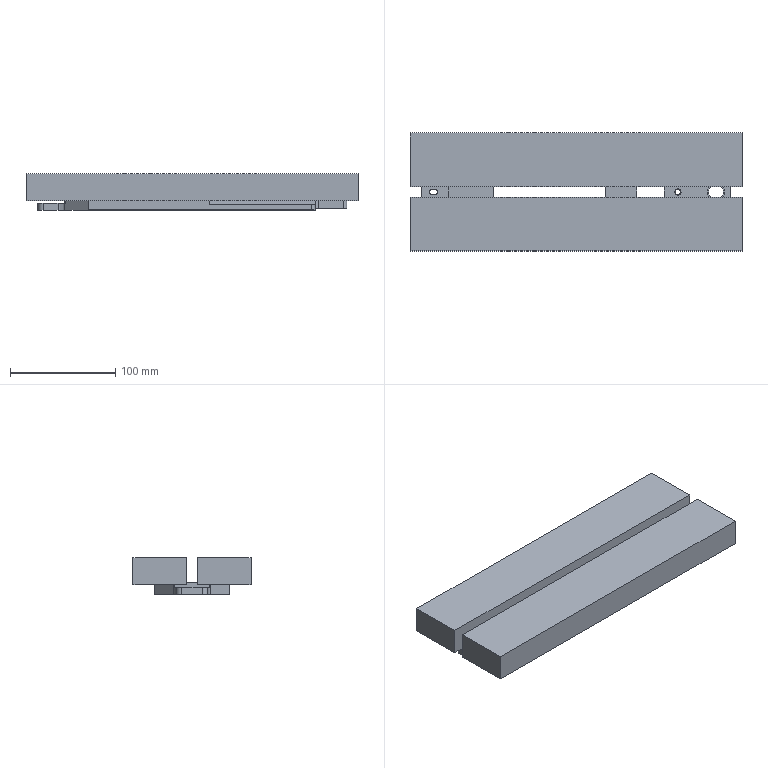NC program | NX | posted with a generic post | part box 315 x 112 x 34.85 mm
Lines 19 to 805 of 11462:
(ADAPTIVE_MILLING , TOOL : D12_ROUGH)
N36 T02 M6
N38 G53
N40 G17 G0 G90 X-161.022 Y-0.963 S6500 M3
N42 G43 Z20. H2
N44 Z-9.
N46 G94 G1 X-160.872 Y-0.957 Z-9.937 F3000.
N48 X-160.722 Y-0.951 Z-10.308
N50 X-160.573 Y-0.945 Z-10.58
N52 X-160.423 Y-0.938 Z-10.8
N54 X-160.273 Y-0.932 Z-10.984
N56 X-160.123 Y-0.926 Z-11.142
N58 X-159.973 Y-0.92 Z-11.28
N60 X-159.823 Y-0.914 Z-11.4
N62 X-159.673 Y-0.908 Z-11.505
N64 X-159.523 Y-0.902 Z-11.598
N66 X-159.374 Y-0.896 Z-11.679
N68 X-159.224 Y-0.89 Z-11.75
N70 X-159.074 Y-0.884 Z-11.81
N72 X-158.924 Y-0.878 Z-11.862
N74 X-158.774 Y-0.872 Z-11.905
N76 X-158.624 Y-0.866 Z-11.939
N78 X-158.474 Y-0.86 Z-11.966
N80 X-158.324 Y-0.854 Z-11.985
N82 X-158.174 Y-0.848 Z-11.996
N84 X-158.025 Y-0.841 Z-12.
N86 X-156.085 Y-0.763
N88 G3 X-155.024 Y-0.037 R1.213
N90 X-154.336 Y3.017 R10.296
N92 X-154.027 Y11.039 R88.268
N94 G1 X-154. Y21.799
N96 G2 X-153.983 Y34.698 R955.634
N98 X-151.786 Y38.926 R6.62
N100 X-146.976 Y41.449 R11.386
N102 X-140.748 Y42.318 R29.799
N104 X-129.951 Y42.495 R232.185
N106 G1 X-123.876 Y42.499
N108 X145.801
N110 G2 X150.265 Y40.486 R6.406
N112 X152.872 Y35.821 R10.892
N114 X153.805 Y29.604 R27.845
N116 X153.995 Y18.207 R225.691
N118 G1 X153.999 Y11.907
N120 X153.998 Y-34.397
N122 G2 X152.106 Y-38.609 R6.376
N124 X147.432 Y-41.316 R10.781
N126 X141.298 Y-42.286 R26.839
N128 X131.476 Y-42.491 R179.768
N130 G1 X123.676 Y-42.499
N132 X-145.826
N134 G2 X-150.172 Y-40.545 R6.379
N136 X-152.866 Y-35.766 R10.949
N138 X-153.801 Y-29.549 R28.01
N140 X-153.994 Y-18.452 R216.598
N142 G1 X-153.999 Y-11.852
N144 X-153.994 Y5.173
N146 G3 X-153.531 Y7.081 R26.231
N148 X-153.077 Y13.66 R49.097
N150 X-152.995 Y31.248 R994.194
N152 G2 X-149.634 Y37.786 R8.754
N154 X-144.116 Y40.403 R14.134
N156 X-136.986 Y41.318 R36.897
N158 X-125.588 Y41.494 R265.971
N160 G1 X-118.988 Y41.499
N162 X-101.337 Y41.5
N164 G3 X-100.411 Y41.826 R2.513
N166 G2 X-98.289 Y42.2 R7.215
N168 G1 X113.711
N170 G2 X116.146 Y41.913 R16.672
N172 G3 X123.066 Y41.545 R62.209
N174 X134.549 Y41.5 R762.557
N176 G2 X143.098 Y41.478 R421.327
N178 X149.417 Y37.997 R8.784
N180 X151.94 Y32.519 R14.268
N182 X152.827 Y25.385 R37.632
N184 X152.995 Y13.987 R280.87
N186 G1 X152.999 Y7.537
N188 X152.997 Y-31.097
N190 G2 X149.622 Y-37.794 R8.752
N192 X144.165 Y-40.39 R14.095
N194 X137.186 Y-41.307 R36.049
N196 X125.339 Y-41.495 R261.794
N198 G1 X117.234 Y-41.511
N200 G3 X116.552 Y-41.75 R3.128
N202 G1 X115.148 Y-42.087
N204 X113.709 Y-42.2
N206 X-98.291
N208 G2 X-100.613 Y-41.898 R21.67
N210 G3 X-107.857 Y-41.539 R67.61
N212 X-119.648 Y-41.5 R794.19
N214 G1 X-142.598 Y-41.498
N216 G2 X-149.284 Y-38.134 R8.75
N218 X-151.91 Y-32.588 R14.151
N220 X-152.811 Y-25.607 R36.598
N222 X-152.993 Y-13.609 R266.033
N224 G1 X-152.999 Y-5.436
N226 G2 X-152.983 Y5.288 R824.874
N228 G3 X-152.49 Y8.476 R39.918
N230 G2 X-152.282 Y12.508 R32.054
N232 G3 X-152.013 Y22.941 R161.961
N234 G2 X-151.969 Y29.075 R201.235
N236 X-147.423 Y36.996 R10.241
N238 X-141.273 Y39.506 R16.877
N240 X-133.453 Y40.345 R46.527
N242 X-118.379 Y40.497 R441.147
N244 G1 X-104.482 Y40.499
N246 G3 X-102.594 Y40.604 R9.216
N248 G1 X-102.277 Y40.748
N250 X-101.391 Y41.369
N252 X-100.847 Y41.622
N254 X-101.391 Y41.369
N256 X-102.395 Y40.654
N258 G2 X-104.258 Y40.192 R5.664
N260 X-110.273 Y39.925 R60.091
N262 G1 X-122.296 Y39.893
N264 G3 X-134.742 Y39.652 R226.868
N266 X-141.852 Y38.604 R34.814
N268 X-147.29 Y35.841 R13.828
N270 X-150.634 Y30.1 R10.73
N272 X-151.308 Y24.374 R29.753
N274 G1 X-151.541 Y15.592
N276 G2 X-151.657 Y14.023 R9.013
N278 G1 X-152.036 Y13.006
N280 X-152.376 Y11.445
N282 X-152.036 Y13.006
N284 G3 X-151.14 Y15.544 R26.474
N286 X-150.538 Y20.465 R29.953
N288 G2 X-150.088 Y26.488 R95.136
N290 X-148.485 Y31.606 R13.365
N292 X-143.036 Y36.419 R12.237
N294 X-136.411 Y38.255 R22.856
N296 X-127.209 Y38.83 R78.815
N298 X-112.541 Y38.913 R971.754
N300 G3 X-105.643 Y39.159 R77.798
N302 X-103.833 Y39.497 R7.727
N304 G1 X-103.609 Y39.629
N306 X-102.288 Y40.739
N308 X-103.782 Y39.486
N310 G2 X-106.184 Y38.756 R6.946
N312 X-112.131 Y38.357 R46.238
N314 X-124.112 Y38.266 R885.684
N316 G3 X-134.15 Y37.857 R115.617
N318 X-140.954 Y36.411 R27.013
N320 X-146.538 Y32.482 R12.6
N322 X-149.081 Y26.769 R14.053
N324 X-149.811 Y21.498 R42.908
N326 G2 X-150.46 Y16.404 R43.199
N328 X-150.711 Y15.906 R1.666
N330 G1 X-151.477 Y14.504
N332 G2 X-150.638 Y16.004 R41.838
N334 G3 X-149.656 Y18.125 R5.692
N336 X-148.735 Y22.918 R47.362
N338 G2 X-147.392 Y28.059 R22.945
N340 X-141.192 Y34.538 R12.717
N342 X-134.538 Y36.537 R22.541
N344 X-125.944 Y37.192 R68.234
N346 X-114.014 Y37.336 R873.961
N348 G3 X-107.369 Y37.716 R57.477
N350 X-105.436 Y38.141 R9.034
N352 G1 X-105.243 Y38.256
N354 X-103.693 Y39.559
N356 X-105.417 Y38.113
N358 G2 X-107.843 Y37.298 R7.378
N360 X-113.764 Y36.79 R40.561
N362 X-124.598 Y36.614 R979.351
N364 G3 X-133.72 Y35.975 R73.644
N366 X-140.245 Y34.068 R22.198
N368 X-146.804 Y26.818 R13.13
N370 X-148.17 Y21.984 R31.33
N372 G2 X-149.256 Y17.819 R31.098
N374 X-149.754 Y17.185 R1.887
N376 G1 X-150.428 Y16.285
N378 G2 X-149.222 Y17.717 R8.221
N380 G3 X-147.996 Y20.064 R7.784
N382 G1 X-146.551 Y24.357
N384 G2 X-143.095 Y30.049 R15.346
N386 X-136.543 Y33.915 R16.052
N388 X-128.886 Y35.307 R34.155
N390 X-118.44 Y35.694 R161.697
N392 G3 X-110.514 Y36.039 R97.198
N394 X-107.222 Y36.656 R16.366
N396 G1 X-106.977 Y36.8
N398 X-105.312 Y38.199
N400 X-107.15 Y36.655
N402 G2 X-109.534 Y35.806 R7.243
N404 X-115.614 Y35.204 R38.765
N406 G3 X-125.866 Y34.878 R827.539
N408 X-133.895 Y33.886 R46.492
N410 X-140.41 Y31.103 R18.239
N412 X-145.287 Y25.101 R15.22
N414 X-147.185 Y20.525 R86.69
N416 G2 X-148.076 Y18.757 R8.533
N418 X-148.624 Y18.315 R6.705
N420 G1 X-149.26 Y17.679
N422 G2 X-147.909 Y18.85 R7.268
N424 G3 X-146.384 Y20.934 R8.025
N426 G2 X-144.143 Y24.995 R97.092
N428 X-135.465 Y31.971 R16.466
N430 X-127.777 Y33.595 R31.965
N432 X-118.897 Y34.088 R132.138
N434 G3 X-111.512 Y34.594 R71.126
N436 X-108.974 Y35.163 R11.718
N438 G1 X-108.784 Y35.282
N440 X-107.118 Y36.681
N442 X-108.956 Y35.137
N444 G2 X-111.543 Y34.22 R7.716
N446 X-117.412 Y33.59 R41.28
N448 G3 X-126.419 Y33.083 R246.05
N450 X-133.999 Y31.676 R35.118
N452 X-143.411 Y24.566 R17.194
N454 X-145.825 Y20.732 R347.167
N456 G2 X-146.652 Y19.668 R5.476
N458 G3 X-147.945 Y18.823 R9.081
N460 G2 X-146.373 Y19.803 R8.108
N462 G3 X-144.494 Y21.681 R9.23
N464 G2 X-141.394 Y25.413 R57.726
N466 X-132.404 Y30.763 R19.687
N468 X-124.284 Y32.138 R41.416
N470 X-116.487 Y32.665 R806.55
N472 G3 X-111.216 Y33.467 R28.558
N474 X-110.647 Y33.717 R1.934
N476 G1 X-108.924 Y35.164
N478 X-110.82 Y33.572
N480 G2 X-113.402 Y32.638 R7.835
N482 X-119.041 Y31.934 R43.599
N484 G3 X-127.086 Y31.181 R120.7
N486 X-134.803 Y29.075 R28.367
N488 X-141.698 Y23.911 R20.858
N490 G2 X-144.537 Y20.793 R86.711
N492 X-145.104 Y20.35 R2.371
N494 G3 X-146.402 Y19.787 R6.455
N496 G2 X-145.104 Y20.35 R6.455
N498 G3 X-143.117 Y21.543 R6.138
N500 G1 X-139.682 Y24.517
N502 G2 X-129.256 Y29.545 R24.551
N504 X-121.918 Y30.642 R57.45
N506 G3 X-115.156 Y31.408 R98.281
N508 X-112.724 Y32.008 R11.913
N510 G1 X-112.559 Y32.111
N512 X-110.778 Y33.607
N514 X-112.731 Y31.967
N516 G2 X-115.4 Y30.983 R8.377
N518 X-120.441 Y30.222 R49.586
N520 G3 X-128.154 Y29.094 R76.929
N522 X-139.68 Y23.566 R26.047
N524 G2 X-142.988 Y20.998 R48.613
N526 G1 X-143.332 Y20.838
N528 G3 X-144.725 Y20.492 R8.423
N530 G2 X-143.332 Y20.838 R8.423
N532 G3 X-140.989 Y21.802 R6.926
N534 G2 X-136.677 Y24.486 R530.565
N536 X-126.061 Y28.318 R32.292
N538 X-118.695 Y29.435 R205.643
N540 G3 X-114.764 Y30.311 R22.958
N542 G1 X-114.557 Y30.433
N544 X-112.719 Y31.977
N546 X-114.73 Y30.29
N548 G2 X-117.28 Y29.292 R8.527
N550 X-122.8 Y28.261 R69.878
N552 G3 X-130.822 Y26.376 R47.603
N554 X-137.85 Y22.977 R36.48
N556 G2 X-141.257 Y21.1 R31.406
N558 G1 X-141.534 Y21.033
N560 X-142.883 Y20.936
N562 G3 X-140.773 Y21.099 R41.743
N564 X-137.648 Y22.245 R14.378
N566 G2 X-131.303 Y25.008 R69.885
N568 X-123.029 Y27.133 R53.867
N570 G3 X-117.436 Y28.347 R59.208
N572 X-116.669 Y28.659 R2.7
N574 G1 X-114.659 Y30.347
N576 X-116.841 Y28.514
N578 G2 X-119.52 Y27.412 R9.596
N580 X-125.615 Y25.979 R178.227
N582 G3 X-135.451 Y22.562 R51.022
N584 G2 X-139.179 Y21.07 R30.883
N586 X-141.202 Y21.05 R28.659
N588 G1 X-138.421 Y21.061
N590 G3 X-135.162 Y21.879 R15.354
N592 G2 X-127.95 Y24.252 R132.533
N594 X-120.997 Y26.028 R482.695
N596 G3 X-119.111 Y26.637 R16.872
N598 G1 X-118.974 Y26.723
N600 X-116.791 Y28.556
N602 G2 X-119.316 Y26.461 R56.651
N604 X-122.413 Y25.198 R13.576
N606 G3 X-129.696 Y23.073 R400.204
N608 G2 X-135.631 Y21.151 R202.756
N610 G1 X-136.109 Y21.05
N612 X-138.584
N614 G3 X-134.618 Y21.07 R118.289
N616 X-130.3 Y21.97 R27.955
N618 X-122.5 Y24.192 R158.808
N620 X-121.482 Y24.616 R4.148
N622 G1 X-119.127 Y26.594
N624 G2 X-121.835 Y24.341 R355.257
N626 X-124.981 Y22.958 R14.335
N628 X-131.71 Y21.056 R73.139
N630 G1 X-134.935 Y21.05
N632 G3 X-129.736 Y21.072 R140.62
N634 X-124.186 Y22.386 R22.572
N636 G1 X-123.996 Y22.504
N638 X-121.641 Y24.482
N640 G2 X-124.358 Y22.226 R82.108
N642 X-127.413 Y21.05 R9.82
N644 G1 X-130.113
N646 X-127.037 Y21.059
N648 G3 X-124.61 Y21.988 R4.123
N650 G1 X-124.151 Y22.374
N652 G3 X-123.887 Y23.9 R1.2
N654 X-124.87 Y24.497 Z-11.949 R1.249
N656 G1 X-126.026 Y24.661 Z-11.9
N658 X-128.591 Y25.023 F15000.
N660 X-128.758 Y25.034
N662 X-139.104
N664 G3 X-146.016 Y23.863 R20.816
N666 X-150.152 Y21.696 R17.213
N668 X-151.834 Y20.369 R14.771
N670 X-154.763 Y16.046 R11.816
N672 G1 X-156.252 Y12.238
N674 G3 X-155.643 Y10.715 R1.2
N676 G1 X-155.419 Y10.61
N678 X-153.277 Y9.608 Z-12. F3000.
N680 G2 X-152.49 Y8.476 R1.229
N682 G1 X-152.48 Y-10.149
N684 G2 X-152.348 Y-20.579 R792.775
N686 G3 X-151.866 Y-28.96 R74.548
N688 X-150.324 Y-34.657 R19.293
N690 X-144.303 Y-39.87 R9.499
N692 X-138.986 Y-40.73 R22.246
N694 X-129.164 Y-40.897 R184.696
N696 G1 X-119.984 Y-40.899
N698 G2 X-105.03 Y-41.019 R488.765
N700 X-101.662 Y-41.263 R40.927
N702 X-100.413 Y-41.825 R13.542
N704 G1 X-99.369 Y-42.105
N706 G2 X-101.74 Y-41.148 R6.88
N708 G3 X-104.831 Y-40.361 R10.23
N710 X-112.369 Y-39.949 R68.231
N712 X-127.374 Y-39.898 R925.483
N714 G2 X-137.497 Y-39.751 R210.096
N716 X-142.526 Y-38.984 R21.206
N718 X-148.456 Y-34.146 R10.547
N720 X-150.592 Y-28.015 R18.309
N722 X-151.279 Y-20.328 R53.766
N724 G1 X-151.4 Y-14.804
N726 X-151.478 Y-14.502
N728 X-152.037 Y-13.004
N730 X-152.376 Y-11.443
N732 X-152.49 Y-9.849
N734 X-152.376 Y-11.443
N736 X-152.037 Y-13.004
N738 G2 X-151.269 Y-15.077 R34.934
N740 X-150.789 Y-19.167 R25.342
N742 G3 X-150.187 Y-26.243 R84.987
N744 X-148.487 Y-32.206 R20.28
N746 X-141.88 Y-37.979 R11.103
N748 X-136.069 Y-39.059 R23.118
N750 X-126.699 Y-39.293 R137.876
N752 G2 X-110.545 Y-39.403 R698.862
N754 X-104.427 Y-39.915 R43.909
N756 X-102.752 Y-40.37 R6.493
N758 G3 X-101.541 Y-41.264 R24.823
N760 G2 X-103.111 Y-40.069 R23.546
N762 G3 X-106.122 Y-39.036 R9.042
N764 X-112.839 Y-38.425 R44.984
N766 X-127.385 Y-38.287 R575.647
N768 G2 X-135.777 Y-37.99 R96.113
N770 X-141.237 Y-36.732 R18.454
N772 X-147.082 Y-31.14 R11.882
N774 X-149.066 Y-24.792 R21.402
N776 X-149.803 Y-18.634 R111.077
N778 G3 X-150.076 Y-16.847 R15.169
N780 X-150.713 Y-15.904 R4.462
N782 G1 X-151.467 Y-14.522
N784 X-150.713 Y-15.904
N786 G2 X-149.973 Y-16.964 R6.486
N788 X-149.179 Y-20.176 R14.162
N790 G3 X-148.165 Y-25.883 R74.214
N792 X-145.773 Y-31.593 R17.068
N794 X-139.473 Y-36.262 R12.338
N796 X-133.073 Y-37.446 R25.387
N798 X-124.153 Y-37.693 R136.558
N800 G2 X-111.916 Y-37.887 R302.115
N802 X-105.767 Y-38.624 R34.417
N804 X-104.177 Y-39.16 R6.673
N806 G1 X-102.967 Y-40.169
N808 X-104.666 Y-38.76
N810 G3 X-107.755 Y-37.604 R9.308
N812 X-114.539 Y-36.874 R41.37
N814 X-126.44 Y-36.667 R433.016
N816 G2 X-134.298 Y-36.21 R66.721
N818 X-140.084 Y-34.47 R17.144
N820 X-145.588 Y-28.586 R13.087
N822 X-147.508 Y-22.835 R26.056
N824 G3 X-148.554 Y-18.563 R55.434
N826 X-148.811 Y-18.128 R2.134
N828 G1 X-149.755 Y-17.184
N830 X-150.159 Y-16.643
N832 X-149.755 Y-17.184
N834 X-148.652 Y-18.288
N836 G2 X-147.617 Y-20.624 R8.394
N838 G3 X-146.097 Y-25.508 R110.553
N840 X-142.81 Y-31.092 R15.93
N842 X-136.479 Y-34.829 R14.029
N844 X-129.676 Y-35.889 R30.789
N846 X-119.627 Y-36.144 R232.539
N848 G2 X-110.681 Y-36.606 R92.849
N850 X-106.073 Y-37.634 R18.877
N852 G1 X-105.811 Y-37.78
N854 X-104.49 Y-38.889
N856 X-106.413 Y-37.294
N858 G3 X-109.707 Y-36.065 R10.028
N860 X-116.446 Y-35.303 R42.3
N862 X-126.502 Y-35.007 R781.633
N864 G2 X-133.657 Y-34.275 R43.226
N866 X-140.047 Y-31.452 R15.174
N868 X-144.388 Y-25.837 R15.718
N870 X-146.357 Y-21.058 R70.404
N872 G3 X-147.091 Y-19.516 R9.302
N874 X-147.436 Y-19.204 R3.133
N876 G2 X-148.731 Y-18.208 R14.158
N878 G3 X-147.216 Y-19.346 R13.904
N880 G2 X-146.016 Y-21.051 R5.891
N882 G3 X-143.983 Y-25.193 R550.573
N884 X-139.676 Y-30.536 R16.172
N886 X-133.087 Y-33.514 R16.608
N888 X-125.872 Y-34.371 R41.661
N890 G2 X-116.382 Y-34.728 R980.335
N892 X-109.787 Y-35.546 R39.858
N894 X-107.676 Y-36.231 R11.21
N896 G1 X-106.251 Y-37.41
N898 G3 X-108.307 Y-35.724 R30.921
N900 X-111.713 Y-34.49 R10.882
N902 X-118.866 Y-33.684 R46.805
N904 G2 X-127.275 Y-33.239 R284.473
N906 X-133.966 Y-31.982 R28.194
N908 X-141.69 Y-26.17 R15.474
N910 X-144.36 Y-21.891 R55.19
N912 G3 X-145.419 Y-20.343 R11.975
N914 X-145.944 Y-20.037 R1.595
N916 G1 X-147.326 Y-19.282
N918 G3 X-145.791 Y-20.094 R18.047
N920 G2 X-144.912 Y-20.732 R2.138
N922 X-142.712 Y-23.653 R25.265
N924 G3 X-138.912 Y-28.102 R22.991
N926 X-131.507 Y-31.791 R17.427
N928 X-124.159 Y-32.784 R42.422
N930 G2 X-115.918 Y-33.326 R244.695
N932 X-110.473 Y-34.327 R27.216
N934 X-109.391 Y-34.773 R4.736
N936 G1 X-108.012 Y-35.93
N938 G3 X-110.116 Y-34.201 R36.319
N940 X-113.491 Y-32.946 R10.93
N942 X-120.113 Y-32.086 R47.614
N944 G2 X-127.488 Y-31.404 R114.947
N946 X-134.243 Y-29.478 R22.815
N948 X-140.131 Y-24.861 R18.805
N950 G3 X-143.037 Y-21.462 R254.56
N952 X-143.915 Y-20.727 R2.685
N954 G2 X-145.711 Y-20.124 R11.729
N956 G1 X-144.446 Y-20.596
N958 G2 X-142.889 Y-21.325 R2.793
N960 X-140.161 Y-23.997 R34.865
N962 G3 X-134.674 Y-28.311 R22.2
N964 X-127.341 Y-30.67 R23.59
N966 X-119.864 Y-31.499 R99.714
N968 G2 X-113.325 Y-32.478 R43.343
N970 X-111.302 Y-33.175 R9.564
N972 G1 X-109.805 Y-34.424
N974 X-111.897 Y-32.686
N976 G3 X-115.228 Y-31.386 R10.708
N978 X-121.291 Y-30.429 R52.249
N980 G2 X-128.328 Y-29.335 R60.074
N982 X-138.059 Y-24.269 R21.966
N984 G3 X-141.312 Y-21.462 R84.644
N986 X-142.232 Y-20.983 R1.959
N988 G2 X-143.911 Y-20.712 R7.581
N990 G3 X-142.008 Y-21.002 R7.682
N992 G2 X-139.973 Y-22.117 R6.827
N994 G3 X-135.998 Y-25.08 R155.16
N996 X-126.598 Y-28.947 R25.023
N998 X-119.663 Y-30.022 R110.783
N1000 G2 X-114.112 Y-31.205 R31.628
N1002 X-113.136 Y-31.626 R4.151
N1004 G1 X-111.701 Y-32.832
N1006 X-113.779 Y-31.101
N1008 G3 X-117.073 Y-29.753 R10.984
N1010 X-123.219 Y-28.541 R79.251
N1012 G2 X-130.525 Y-26.585 R36.214
N1014 X-136.622 Y-23.186 R31.705
N1016 G3 X-139.837 Y-21.154 R30.214
N1018 X-140.273 Y-21.05 R3.512
N1020 G2 X-142.113 Y-20.991 R16.35
N1022 G3 X-140.048 Y-21.052 R18.13
N1024 G2 X-137.715 Y-22.001 R7.834
N1026 G3 X-133.127 Y-24.606 R161.037
N1028 X-124.133 Y-27.676 R34.358
N1030 G2 X-117.887 Y-28.992 R159.303
N1032 X-115.221 Y-29.892 R15.746
N1034 G1 X-113.631 Y-31.211
N1036 X-115.831 Y-29.38
N1038 G3 X-119.248 Y-27.932 R12.7
N1040 X-125.11 Y-26.415 R292.167
N1042 G2 X-134.073 Y-22.804 R39.74
N1044 G3 X-137.517 Y-21.097 R34.866
N1046 G1 X-137.795 Y-21.05
N1048 X-140.195
N1050 X-137.57
N1052 G2 X-134.976 Y-21.872 R9.659
N1054 G3 X-129.268 Y-24.349 R124.539
N1056 X-121.8 Y-26.617 R72.218
N1058 G2 X-117.428 Y-28.052 R29.908
N1060 X-115.674 Y-29.495 R25.482
N1062 G1 X-118.051 Y-27.514
N1064 G3 X-121.36 Y-25.967 R14.651
N1066 G2 X-127.859 Y-23.741 R313.913
N1068 X-133.799 Y-21.311 R326.478
N1070 G3 X-134.664 Y-21.05 R3.272
N1072 G1 X-137.589
N1074 X-134.236 Y-21.065
N1076 G2 X-130.978 Y-21.972 R16.151
N1078 G3 X-121.948 Y-25.15 R579.551
N1080 G2 X-119.726 Y-26.091 R14.742
N1082 G1 X-117.889 Y-27.634
N1084 X-120.678 Y-25.308
N1086 G3 X-124.263 Y-23.496 R19.531
N1088 X-130.707 Y-21.079 R97.175
N1090 G1 X-130.917 Y-21.05
N1092 X-134.442
N1094 X-130.384 Y-21.066
N1096 G2 X-126.589 Y-22.048 R18.189
N1098 X-122.57 Y-23.703 R29.343
N1100 G1 X-120.487 Y-25.452
N1102 X-123.596 Y-22.853
N1104 G3 X-127.243 Y-21.07 R14.131
N1106 G1 X-127.392 Y-21.05
N1108 X-130.617
N1110 X-127.039 Y-21.059
N1112 G2 X-125.262 Y-21.549 R6.448
N1114 X-123.463 Y-22.952 R14.108
N1116 G3 X-125.281 Y-21.536 R14.11
N1118 X-126.828 Y-21.083 R3.539
N1120 X-127.989 Y-21.633 R1.213
N1122 G1 X-128.242 Y-22.022
N1124 X-128.48 Y-22.421
N1126 G3 X-127.912 Y-24.014 R1.212
N1128 G1 X-127.778 Y-24.08 Z-11.996
N1130 X-127.643 Y-24.146 Z-11.985
N1132 X-127.509 Y-24.212 Z-11.966
N1134 X-127.374 Y-24.278 Z-11.939
N1136 X-127.239 Y-24.344 Z-11.905
N1138 X-127.105 Y-24.411 Z-11.862
N1140 X-126.97 Y-24.477 Z-11.81
N1142 X-126.835 Y-24.543 Z-11.75
N1144 X-126.701 Y-24.609 Z-11.679
N1146 X-126.566 Y-24.675 Z-11.598
N1148 X-126.432 Y-24.741 Z-11.505
N1150 X-126.297 Y-24.807 Z-11.4
N1152 X-126.162 Y-24.874 Z-11.28
N1154 X-126.028 Y-24.94 Z-11.142
N1156 X-125.893 Y-25.006 Z-10.984
N1158 X-125.758 Y-25.072 Z-10.8
N1160 X-125.624 Y-25.138 Z-10.58
N1162 X-125.489 Y-25.204 Z-10.308
N1164 X-125.354 Y-25.27 Z-9.937
N1166 X-125.22 Y-25.336 Z-9.
N1168 G0 Z20.
N1170 X111.275 Y46.658
N1172 Z-9.
N1174 G1 X111.404 Y46.582 Z-9.937
N1176 X111.534 Y46.507 Z-10.308
N1178 X111.664 Y46.432 Z-10.58
N1180 X111.793 Y46.356 Z-10.8
N1182 X111.923 Y46.281 Z-10.984
N1184 X112.053 Y46.205 Z-11.142
N1186 X112.182 Y46.13 Z-11.28
N1188 X112.312 Y46.054 Z-11.4
N1190 X112.442 Y45.979 Z-11.505
N1192 X112.571 Y45.904 Z-11.598
N1194 X112.701 Y45.828 Z-11.679
N1196 X112.831 Y45.753 Z-11.75
N1198 X112.96 Y45.677 Z-11.81
N1200 X113.09 Y45.602 Z-11.862
N1202 X113.22 Y45.527 Z-11.905
N1204 X113.349 Y45.451 Z-11.939
N1206 X113.479 Y45.376 Z-11.966
N1208 X113.609 Y45.3 Z-11.985
N1210 X113.738 Y45.225 Z-11.996
N1212 X113.868 Y45.15 Z-12.
N1214 G2 X114.457 Y43.923 R1.212
N1216 G1 X114.404 Y43.586
N1218 X114.367 Y43.246
N1220 G3 X115.296 Y42.051 R1.212
N1222 G1 X116.554 Y41.749
N1224 G3 X119.714 Y40.954 R10.823
N1226 X126.976 Y40.554 R68.07
N1228 X140.174 Y40.489 R910.158
N1230 G2 X148.531 Y35.894 R10.245
N1232 X150.977 Y29.941 R16.745
N1234 X151.834 Y22.273 R44.766
N1236 X151.994 Y13.584 R306.51
N1238 G1 X152.054 Y13.323
N1240 X152.46 Y12.342
N1242 X152.797 Y10.938
N1244 X152.91 Y9.499
N1246 Y-9.501
N1248 X152.796 Y-10.94
N1250 G3 X152.194 Y-15.134 R19.308
N1252 X152.004 Y-25.481 R197.861
N1254 G2 X151.938 Y-29.449 R52.579
N1256 X147.516 Y-36.927 R10.222
N1258 X141.388 Y-39.479 R16.671
N1260 X133.645 Y-40.337 R45.315
N1262 X119.839 Y-40.503 R406.017
N1264 G3 X118.734 Y-40.678 R2.348
N1266 G2 X116.985 Y-41.571 R7.303
N1268 G3 X118.862 Y-40.6 R8.076
N1270 G2 X120.759 Y-40.169 R6.117
N1272 X127.013 Y-39.891 R73.159
N1274 G3 X136.527 Y-39.514 R130.692
N1276 X143.061 Y-38.22 R27.222
N1278 X148.297 Y-34.832 R12.172
N1280 X150.753 Y-29.592 R11.44
N1282 X151.341 Y-23.553 R35.643
N1284 G2 X151.619 Y-15.371 R228.485
N1286 X151.783 Y-13.935 R8.112
N1288 G1 X152.459 Y-12.344
N1290 X152.547 Y-11.979
N1292 X152.459 Y-12.344
N1294 X151.865 Y-13.746
N1296 G3 X151.057 Y-15.958 R6.135
N1298 X150.512 Y-20.977 R37.748
N1300 G2 X150.048 Y-26.789 R74.276
N1302 X148.162 Y-32.123 R12.653
N1304 X142.528 Y-36.647 R12.644
N1306 X135.86 Y-38.328 R24.508
N1308 X127.779 Y-38.845 R87.917
N1310 G3 X121.622 Y-39.187 R69.133
N1312 X120.33 Y-39.459 R5.148
N1314 G1 X120.126 Y-39.581
N1316 X119.117 Y-40.444
N1318 X118.861 Y-40.6
N1320 X119.117 Y-40.444
N1322 X120.272 Y-39.458
N1324 G2 X122.619 Y-38.731 R6.741
N1326 X128.237 Y-38.259 R53.239
N1328 G3 X136.082 Y-37.621 R78.888
N1330 X142.328 Y-35.817 R21.451
N1332 X148.608 Y-28.512 R11.925
N1334 X149.69 Y-22.774 R27.534
N1336 G2 X150.305 Y-17.251 R94.23
N1338 X150.734 Y-15.456 R9.661
N1340 X151.152 Y-14.909 R3.238
N1342 G1 X151.701 Y-14.013
N1344 G2 X150.61 Y-15.544 R7.257
N1346 G3 X149.57 Y-18.14 R7.849
N1348 X148.654 Y-23.325 R77.28
N1350 G2 X147.19 Y-28.507 R20.251
N1352 X141.146 Y-34.56 R12.785
N1354 X134.416 Y-36.567 R23.029
N1356 X126.822 Y-37.318 R99.929
N1358 G3 X122.134 Y-38.008 R26.041
N1360 X121.066 Y-38.509 R2.308
N1362 G1 X120.214 Y-39.506
N1364 X121.202 Y-38.353
N1366 G2 X123.316 Y-37.419 R5.615
N1368 X128.158 Y-36.671 R33.632
N1370 G3 X134.84 Y-35.811 R75.579
N1372 X141.175 Y-33.569 R19.943
N1374 X146.778 Y-26.871 R13.104
N1376 X148.18 Y-21.819 R30.616
N1378 G2 X149.286 Y-17.378 R34.34
N1380 X149.831 Y-16.334 R2.715
N1382 G3 X150.653 Y-15.493 R4.213
N1384 G2 X149.546 Y-16.577 R6.02
N1386 G3 X148.257 Y-18.871 R6.846
N1388 X146.877 Y-23.254 R87.323
N1390 G2 X144.42 Y-28.463 R18.008
N1392 X137.98 Y-33.401 R14.691
N1394 X131.32 Y-35.146 R29.445
N1396 G3 X125.43 Y-36.051 R201.787
N1398 X122.101 Y-37.109 R11.81
N1400 X121.727 Y-37.471 R1.973
N1402 G1 X121.152 Y-38.409
N1404 X121.846 Y-37.28
N1406 G2 X123.493 Y-36.251 R4.407
N1408 X127.762 Y-35.157 R21.993
N1410 G3 X133.985 Y-33.945 R85.733
N1412 X140.288 Y-31.2 R19.108
N1414 X145.245 Y-25.093 R15.007
N1416 X147.137 Y-20.228 R62.155
N1418 G2 X148.477 Y-17.416 R13.322
N1420 X149.117 Y-16.944 R2.269
N1422 G1 X149.573 Y-16.554
N1424 G2 X148.417 Y-17.372 R5.576
N1426 G3 X146.998 Y-19.175 R6.195
N1428 X145.042 Y-23.145 R73.431
N1430 G2 X141.237 Y-28.513 R18.07
N1432 X134.662 Y-32.332 R18.113
N1434 X128.389 Y-33.959 R54.858
N1436 G3 X123.91 Y-35.247 R26.118
N1438 X122.432 Y-36.108 R4.782
N1440 G1 X122.222 Y-36.418
N1442 G2 X121.789 Y-37.37 R4.705
N1444 G3 X122.31 Y-36.211 R7.494
N1446 G2 X123.847 Y-34.991 R4.07
N1448 X127.93 Y-33.555 R20.03
N1450 G3 X133.833 Y-31.888 R76.021
N1452 X140.497 Y-27.981 R18.334
N1454 X144.293 Y-22.889 R20.786
N1456 G2 X146.502 Y-19.008 R60.851
N1458 X147.38 Y-17.938 R4.565
N1460 X147.886 Y-17.698 R6.359
N1462 G1 X148.461 Y-17.345
N1464 G2 X147.284 Y-17.947 R4.936
N1466 G3 X145.528 Y-19.584 R5.919
N1468 X143.061 Y-23.101 R90.627
N1470 G2 X133.631 Y-30.558 R20.003
N1472 X127.914 Y-32.479 R75.24
N1474 G3 X123.815 Y-34.168 R19.83
N1476 X122.75 Y-35.009 R3.788
N1478 X122.459 Y-35.844 R2.119
N1480 G1 X122.258 Y-36.329
N1482 G3 X122.631 Y-35.149 R5.206
N1484 G2 X123.859 Y-33.869 R3.544
N1486 X127.567 Y-32.095 R16.46
N1488 G3 X133.07 Y-30.065 R113.582
N1490 X141.966 Y-23.279 R21.276
N1492 G2 X144.802 Y-19.633 R151.424
N1494 X146.081 Y-18.404 R6.118
N1496 X146.552 Y-18.25 R3.098
N1498 G1 X147.314 Y-17.934
N1500 G2 X146.011 Y-18.38 R4.963
N1502 G3 X144.106 Y-19.673 R5.772
N1504 X140.957 Y-22.988 R86.881
N1506 G2 X131.926 Y-29.221 R26.181
N1508 G3 X126.589 Y-31.443 R526.336
N1510 X123.421 Y-33.359 R12.667
N1512 X122.796 Y-34.44 R1.53
N1514 G1 X122.604 Y-35.243
N1516 G3 X122.826 Y-34.113 R4.989
N1518 G2 X123.694 Y-32.868 R2.827
N1520 X126.846 Y-30.848 R12.918
N1522 G1 X132.173 Y-28.415
N1524 G3 X140.626 Y-22.307 R29.232
N1526 G2 X143.799 Y-19.287 R42.122
N1528 X144.891 Y-18.62 R3.228
N1530 G3 X146.023 Y-18.377 R10.344
N1532 G2 X144.706 Y-18.622 R5.787
N1534 G3 X142.623 Y-19.632 R5.673
N1536 X139.061 Y-22.517 R57.468
N1538 G2 X130.438 Y-27.992 R39.803
N1540 G3 X125.639 Y-30.478 R57.421
N1542 X123.101 Y-32.63 R8.946
N1544 X122.896 Y-33.174 R1.654
N1546 G1 X122.814 Y-34.221
N1548 X122.92 Y-32.926
N1550 G2 X124.057 Y-31.285 R4.006
N1552 X127.513 Y-28.904 R16.685
N1554 G3 X133.179 Y-25.828 R205.224
N1556 X138.92 Y-21.776 R47.542
N1558 G2 X142.496 Y-19.152 R31.016
N1560 X143.599 Y-18.7 R2.737
N1562 G1 X144.756 Y-18.618
N1564 G2 X143.044 Y-18.722 R64.228
N1566 G3 X140.456 Y-19.812 R7.964
N1568 X135.789 Y-22.921 R127.589
N1570 G2 X128.64 Y-27.14 R98.696
N1572 G3 X124.541 Y-29.848 R25.678
N1574 X123.017 Y-31.601 R6.599
N1576 X122.91 Y-32.036 R3.664
N1578 G1 Y-33.001
N1580 X122.914 Y-31.811
N1582 G2 X123.923 Y-30.068 R3.978
N1584 X127.407 Y-27.306 R16.418
N1586 G1 X133.487 Y-23.647
N1588 X138.825 Y-20.168
N1590 G2 X141.656 Y-18.735 R14.165
N1592 G1 X141.878 Y-18.7
N1594 X143.228
N1596 G3 X141.169 Y-18.719 R43.333
N1598 X138.153 Y-19.814 R9.998
N1600 X132.571 Y-23.05 R112.864
N1602 X126.62 Y-26.724 R103.763